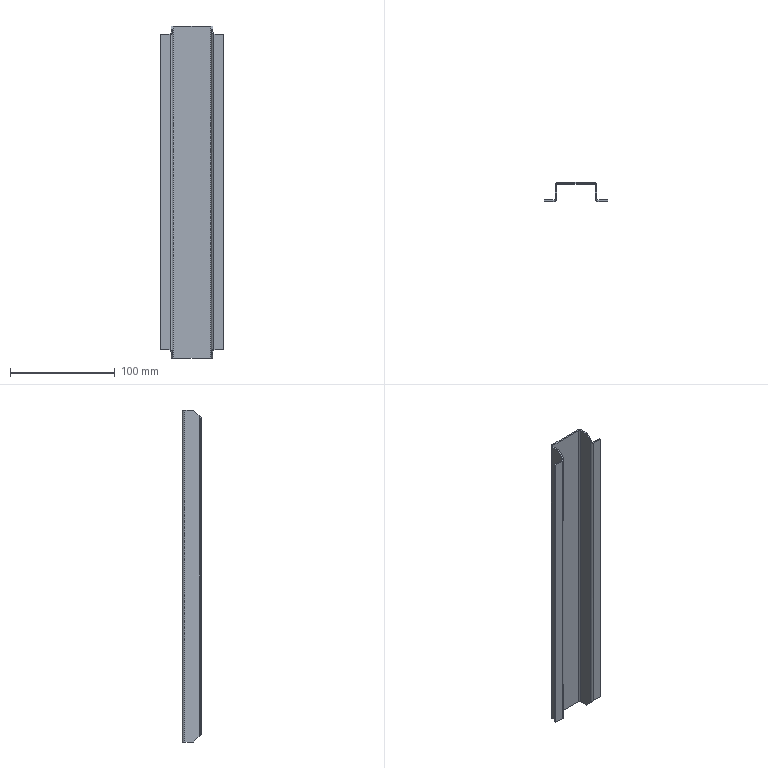Part | SolidWorks | features FlatPattern 1, ICE 1, SMBaseFlange 1, SheetMetal 1 | 1 solid | 42 faces | box 61 x 18.5 x 317 mm | volume 43080 mm3 | plane 30 | cylinder 8 | spline 4 | commonest cylinder face diameters 2 x4 5 x4
STEP:
#1=CARTESIAN_POINT('',(22.477,26.708,8.));
#2=VERTEX_POINT('',#1);
#3=CARTESIAN_POINT('',(12.977,26.708,8.));
#4=VERTEX_POINT('',#3);
#5=CARTESIAN_POINT('',(168.477,26.708,8.));
#6=DIRECTION('',(-1.,0.,0.));
#7=VECTOR('',#6,1000.);
#8=LINE('',#5,#7);
#9=EDGE_CURVE('',#2,#4,#8,.T.);
#10=ORIENTED_EDGE('',*,*,#9,.F.);
#11=CARTESIAN_POINT('',(22.477,26.708,309.));
#12=VERTEX_POINT('',#11);
#13=CARTESIAN_POINT('',(22.477,26.708,317.));
#14=DIRECTION('',(0.,0.,-1.));
#15=VECTOR('',#14,1000.);
#16=LINE('',#13,#15);
#17=EDGE_CURVE('',#12,#2,#16,.T.);
#18=ORIENTED_EDGE('',*,*,#17,.F.);
#19=CARTESIAN_POINT('',(12.977,26.708,309.));
#20=VERTEX_POINT('',#19);
#21=CARTESIAN_POINT('',(168.477,26.708,309.));
#22=DIRECTION('',(-1.,0.,0.));
#23=VECTOR('',#22,1000.);
#24=LINE('',#21,#23);
#25=EDGE_CURVE('',#12,#20,#24,.T.);
#26=ORIENTED_EDGE('',*,*,#25,.T.);
#27=CARTESIAN_POINT('',(12.977,26.708,317.));
#28=DIRECTION('',(0.,0.,-1.));
#29=VECTOR('',#28,1000.);
#30=LINE('',#27,#29);
#31=EDGE_CURVE('',#20,#4,#30,.T.);
#32=ORIENTED_EDGE('',*,*,#31,.T.);
#33=EDGE_LOOP('',(#10,#18,#26,#32));
#34=FACE_OUTER_BOUND('',#33,.T.);
#35=CARTESIAN_POINT('',(11.977,26.708,317.));
#36=DIRECTION('',(0.,1.,0.));
#37=DIRECTION('',(0.,0.,1.));
#38=AXIS2_PLACEMENT_3D('',#35,#36,#37);
#39=PLANE('',#38);
#40=ADVANCED_FACE('',(#34),#39,.F.);
#41=ORIENTED_EDGE('',*,*,#17,.T.);
#42=CARTESIAN_POINT('',(22.477,28.208,8.));
#43=VERTEX_POINT('',#42);
#44=CARTESIAN_POINT('',(22.477,26.708,8.));
#45=DIRECTION('',(0.,1.,0.));
#46=VECTOR('',#45,1000.);
#47=LINE('',#44,#46);
#48=EDGE_CURVE('',#2,#43,#47,.T.);
#49=ORIENTED_EDGE('',*,*,#48,.T.);
#50=CARTESIAN_POINT('',(22.477,28.208,309.));
#51=VERTEX_POINT('',#50);
#52=CARTESIAN_POINT('',(22.477,28.208,317.));
#53=DIRECTION('',(0.,0.,-1.));
#54=VECTOR('',#53,1000.);
#55=LINE('',#52,#54);
#56=EDGE_CURVE('',#51,#43,#55,.T.);
#57=ORIENTED_EDGE('',*,*,#56,.F.);
#58=CARTESIAN_POINT('',(22.477,26.708,309.));
#59=DIRECTION('',(0.,1.,0.));
#60=VECTOR('',#59,1000.);
#61=LINE('',#58,#60);
#62=EDGE_CURVE('',#12,#51,#61,.T.);
#63=ORIENTED_EDGE('',*,*,#62,.F.);
#64=EDGE_LOOP('',(#41,#49,#57,#63));
#65=FACE_OUTER_BOUND('',#64,.T.);
#66=CARTESIAN_POINT('',(22.477,28.208,317.));
#67=DIRECTION('',(1.,0.,0.));
#68=DIRECTION('',(0.,0.,-1.));
#69=AXIS2_PLACEMENT_3D('',#66,#67,#68);
#70=PLANE('',#69);
#71=ADVANCED_FACE('',(#65),#70,.T.);
#72=ORIENTED_EDGE('',*,*,#56,.T.);
#73=CARTESIAN_POINT('',(12.977,28.208,8.));
#74=VERTEX_POINT('',#73);
#75=CARTESIAN_POINT('',(11.977,28.208,8.));
#76=DIRECTION('',(-1.,0.,0.));
#77=VECTOR('',#76,1000.);
#78=LINE('',#75,#77);
#79=EDGE_CURVE('',#43,#74,#78,.T.);
#80=ORIENTED_EDGE('',*,*,#79,.T.);
#81=CARTESIAN_POINT('',(12.977,28.208,309.));
#82=VERTEX_POINT('',#81);
#83=CARTESIAN_POINT('',(12.977,28.208,317.));
#84=DIRECTION('',(0.,0.,-1.));
#85=VECTOR('',#84,1000.);
#86=LINE('',#83,#85);
#87=EDGE_CURVE('',#82,#74,#86,.T.);
#88=ORIENTED_EDGE('',*,*,#87,.F.);
#89=CARTESIAN_POINT('',(11.977,28.208,309.));
#90=DIRECTION('',(-1.,0.,0.));
#91=VECTOR('',#90,1000.);
#92=LINE('',#89,#91);
#93=EDGE_CURVE('',#51,#82,#92,.T.);
#94=ORIENTED_EDGE('',*,*,#93,.F.);
#95=EDGE_LOOP('',(#72,#80,#88,#94));
#96=FACE_OUTER_BOUND('',#95,.T.);
#97=CARTESIAN_POINT('',(11.977,28.208,317.));
#98=DIRECTION('',(0.,1.,0.));
#99=DIRECTION('',(0.,0.,1.));
#100=AXIS2_PLACEMENT_3D('',#97,#98,#99);
#101=PLANE('',#100);
#102=ADVANCED_FACE('',(#96),#101,.T.);
#103=ORIENTED_EDGE('',*,*,#87,.T.);
#104=CARTESIAN_POINT('',(11.977,29.208,5.5));
#105=VERTEX_POINT('',#104);
#106=CARTESIAN_POINT('',(11.977,29.208,5.5));
#107=CARTESIAN_POINT('',(11.977,28.623,6.964));
#108=CARTESIAN_POINT('',(12.391,28.208,8.));
#109=CARTESIAN_POINT('',(12.977,28.208,8.));
#110=(BOUNDED_CURVE()B_SPLINE_CURVE(3,(#106,#107,#108,#109),.UNSPECIFIED.,.F.,.F.)B_SPLINE_CURVE_WITH_KNOTS((4,4),(1.571,3.142),.UNSPECIFIED.)CURVE()GEOMETRIC_REPRESENTATION_ITEM()RATIONAL_B_SPLINE_CURVE((1.,0.8047,0.8047,1.))REPRESENTATION_ITEM(''));
#111=EDGE_CURVE('',#105,#74,#110,.T.);
#112=ORIENTED_EDGE('',*,*,#111,.F.);
#113=CARTESIAN_POINT('',(11.977,29.208,311.5));
#114=VERTEX_POINT('',#113);
#115=CARTESIAN_POINT('',(11.977,29.208,317.));
#116=DIRECTION('',(0.,0.,-1.));
#117=VECTOR('',#116,1000.);
#118=LINE('',#115,#117);
#119=EDGE_CURVE('',#114,#105,#118,.T.);
#120=ORIENTED_EDGE('',*,*,#119,.F.);
#121=CARTESIAN_POINT('',(12.977,28.208,309.));
#122=CARTESIAN_POINT('',(12.391,28.208,309.));
#123=CARTESIAN_POINT('',(11.977,28.623,310.036));
#124=CARTESIAN_POINT('',(11.977,29.208,311.5));
#125=(BOUNDED_CURVE()B_SPLINE_CURVE(3,(#121,#122,#123,#124),.UNSPECIFIED.,.F.,.F.)B_SPLINE_CURVE_WITH_KNOTS((4,4),(0.,1.571),.UNSPECIFIED.)CURVE()GEOMETRIC_REPRESENTATION_ITEM()RATIONAL_B_SPLINE_CURVE((1.,0.8047,0.8047,1.))REPRESENTATION_ITEM(''));
#126=EDGE_CURVE('',#82,#114,#125,.T.);
#127=ORIENTED_EDGE('',*,*,#126,.F.);
#128=EDGE_LOOP('',(#103,#112,#120,#127));
#129=FACE_OUTER_BOUND('',#128,.T.);
#130=CARTESIAN_POINT('',(12.977,29.208,317.));
#131=DIRECTION('',(0.,0.,-1.));
#132=DIRECTION('',(-1.,0.,0.));
#133=AXIS2_PLACEMENT_3D('',#130,#131,#132);
#134=CYLINDRICAL_SURFACE('',#133,1.);
#135=ADVANCED_FACE('',(#129),#134,.F.);
#136=ORIENTED_EDGE('',*,*,#119,.T.);
#137=CARTESIAN_POINT('',(11.977,34.708,0.));
#138=VERTEX_POINT('',#137);
#139=CARTESIAN_POINT('',(11.977,-118.542,153.25));
#140=DIRECTION('',(0.,-0.7071,0.7071));
#141=VECTOR('',#140,1000.);
#142=LINE('',#139,#141);
#143=EDGE_CURVE('',#138,#105,#142,.T.);
#144=ORIENTED_EDGE('',*,*,#143,.F.);
#145=CARTESIAN_POINT('',(11.977,42.708,0.));
#146=VERTEX_POINT('',#145);
#147=CARTESIAN_POINT('',(11.977,45.208,0.));
#148=DIRECTION('',(0.,-1.,0.));
#149=VECTOR('',#148,1000.);
#150=LINE('',#147,#149);
#151=EDGE_CURVE('',#146,#138,#150,.T.);
#152=ORIENTED_EDGE('',*,*,#151,.F.);
#153=CARTESIAN_POINT('',(11.977,42.708,317.));
#154=VERTEX_POINT('',#153);
#155=CARTESIAN_POINT('',(11.977,42.708,317.));
#156=DIRECTION('',(0.,0.,-1.));
#157=VECTOR('',#156,1000.);
#158=LINE('',#155,#157);
#159=EDGE_CURVE('',#154,#146,#158,.T.);
#160=ORIENTED_EDGE('',*,*,#159,.F.);
#161=CARTESIAN_POINT('',(11.977,34.708,317.));
#162=VERTEX_POINT('',#161);
#163=CARTESIAN_POINT('',(11.977,45.208,317.));
#164=DIRECTION('',(0.,-1.,0.));
#165=VECTOR('',#164,1000.);
#166=LINE('',#163,#165);
#167=EDGE_CURVE('',#154,#162,#166,.T.);
#168=ORIENTED_EDGE('',*,*,#167,.T.);
#169=CARTESIAN_POINT('',(11.977,39.958,322.25));
#170=DIRECTION('',(0.,0.7071,0.7071));
#171=VECTOR('',#170,1000.);
#172=LINE('',#169,#171);
#173=EDGE_CURVE('',#114,#162,#172,.T.);
#174=ORIENTED_EDGE('',*,*,#173,.F.);
#175=EDGE_LOOP('',(#136,#144,#152,#160,#168,#174));
#176=FACE_OUTER_BOUND('',#175,.T.);
#177=CARTESIAN_POINT('',(11.977,45.208,317.));
#178=DIRECTION('',(1.,0.,0.));
#179=DIRECTION('',(0.,0.,-1.));
#180=AXIS2_PLACEMENT_3D('',#177,#178,#179);
#181=PLANE('',#180);
#182=ADVANCED_FACE('',(#176),#181,.T.);
#183=CARTESIAN_POINT('',(10.477,34.708,0.));
#184=VERTEX_POINT('',#183);
#185=CARTESIAN_POINT('',(10.477,29.208,5.5));
#186=VERTEX_POINT('',#185);
#187=CARTESIAN_POINT('',(10.477,-118.542,153.25));
#188=DIRECTION('',(0.,-0.7071,0.7071));
#189=VECTOR('',#188,1000.);
#190=LINE('',#187,#189);
#191=EDGE_CURVE('',#184,#186,#190,.T.);
#192=ORIENTED_EDGE('',*,*,#191,.T.);
#193=CARTESIAN_POINT('',(10.477,29.208,311.5));
#194=VERTEX_POINT('',#193);
#195=CARTESIAN_POINT('',(10.477,29.208,317.));
#196=DIRECTION('',(0.,0.,-1.));
#197=VECTOR('',#196,1000.);
#198=LINE('',#195,#197);
#199=EDGE_CURVE('',#194,#186,#198,.T.);
#200=ORIENTED_EDGE('',*,*,#199,.F.);
#201=CARTESIAN_POINT('',(10.477,34.708,317.));
#202=VERTEX_POINT('',#201);
#203=CARTESIAN_POINT('',(10.477,39.958,322.25));
#204=DIRECTION('',(0.,0.7071,0.7071));
#205=VECTOR('',#204,1000.);
#206=LINE('',#203,#205);
#207=EDGE_CURVE('',#194,#202,#206,.T.);
#208=ORIENTED_EDGE('',*,*,#207,.T.);
#209=CARTESIAN_POINT('',(10.477,42.708,317.));
#210=VERTEX_POINT('',#209);
#211=CARTESIAN_POINT('',(10.477,45.208,317.));
#212=DIRECTION('',(0.,-1.,0.));
#213=VECTOR('',#212,1000.);
#214=LINE('',#211,#213);
#215=EDGE_CURVE('',#210,#202,#214,.T.);
#216=ORIENTED_EDGE('',*,*,#215,.F.);
#217=CARTESIAN_POINT('',(10.477,42.708,0.));
#218=VERTEX_POINT('',#217);
#219=CARTESIAN_POINT('',(10.477,42.708,317.));
#220=DIRECTION('',(0.,0.,-1.));
#221=VECTOR('',#220,1000.);
#222=LINE('',#219,#221);
#223=EDGE_CURVE('',#210,#218,#222,.T.);
#224=ORIENTED_EDGE('',*,*,#223,.T.);
#225=CARTESIAN_POINT('',(10.477,45.208,0.));
#226=DIRECTION('',(0.,-1.,0.));
#227=VECTOR('',#226,1000.);
#228=LINE('',#225,#227);
#229=EDGE_CURVE('',#218,#184,#228,.T.);
#230=ORIENTED_EDGE('',*,*,#229,.T.);
#231=EDGE_LOOP('',(#192,#200,#208,#216,#224,#230));
#232=FACE_OUTER_BOUND('',#231,.T.);
#233=CARTESIAN_POINT('',(10.477,45.208,317.));
#234=DIRECTION('',(1.,0.,0.));
#235=DIRECTION('',(0.,0.,-1.));
#236=AXIS2_PLACEMENT_3D('',#233,#234,#235);
#237=PLANE('',#236);
#238=ADVANCED_FACE('',(#232),#237,.F.);
#239=CARTESIAN_POINT('',(10.477,29.208,5.5));
#240=CARTESIAN_POINT('',(10.477,27.744,6.964));
#241=CARTESIAN_POINT('',(11.512,26.708,8.));
#242=CARTESIAN_POINT('',(12.977,26.708,8.));
#243=(BOUNDED_CURVE()B_SPLINE_CURVE(3,(#239,#240,#241,#242),.UNSPECIFIED.,.F.,.F.)B_SPLINE_CURVE_WITH_KNOTS((4,4),(1.571,3.142),.UNSPECIFIED.)CURVE()GEOMETRIC_REPRESENTATION_ITEM()RATIONAL_B_SPLINE_CURVE((1.,0.8047,0.8047,1.))REPRESENTATION_ITEM(''));
#244=EDGE_CURVE('',#186,#4,#243,.T.);
#245=ORIENTED_EDGE('',*,*,#244,.T.);
#246=ORIENTED_EDGE('',*,*,#31,.F.);
#247=CARTESIAN_POINT('',(12.977,26.708,309.));
#248=CARTESIAN_POINT('',(11.512,26.708,309.));
#249=CARTESIAN_POINT('',(10.477,27.744,310.036));
#250=CARTESIAN_POINT('',(10.477,29.208,311.5));
#251=(BOUNDED_CURVE()B_SPLINE_CURVE(3,(#247,#248,#249,#250),.UNSPECIFIED.,.F.,.F.)B_SPLINE_CURVE_WITH_KNOTS((4,4),(0.,1.571),.UNSPECIFIED.)CURVE()GEOMETRIC_REPRESENTATION_ITEM()RATIONAL_B_SPLINE_CURVE((1.,0.8047,0.8047,1.))REPRESENTATION_ITEM(''));
#252=EDGE_CURVE('',#20,#194,#251,.T.);
#253=ORIENTED_EDGE('',*,*,#252,.T.);
#254=ORIENTED_EDGE('',*,*,#199,.T.);
#255=EDGE_LOOP('',(#245,#246,#253,#254));
#256=FACE_OUTER_BOUND('',#255,.T.);
#257=CARTESIAN_POINT('',(12.977,29.208,317.));
#258=DIRECTION('',(0.,0.,-1.));
#259=DIRECTION('',(-1.,0.,0.));
#260=AXIS2_PLACEMENT_3D('',#257,#258,#259);
#261=CYLINDRICAL_SURFACE('',#260,2.5);
#262=ADVANCED_FACE('',(#256),#261,.T.);
#263=CARTESIAN_POINT('',(-28.023,34.708,0.));
#264=VERTEX_POINT('',#263);
#265=CARTESIAN_POINT('',(-28.023,42.708,0.));
#266=VERTEX_POINT('',#265);
#267=CARTESIAN_POINT('',(-28.023,28.208,0.));
#268=DIRECTION('',(0.,1.,0.));
#269=VECTOR('',#268,1000.);
#270=LINE('',#267,#269);
#271=EDGE_CURVE('',#264,#266,#270,.T.);
#272=ORIENTED_EDGE('',*,*,#271,.F.);
#273=CARTESIAN_POINT('',(-28.023,29.208,5.5));
#274=VERTEX_POINT('',#273);
#275=CARTESIAN_POINT('',(-28.023,-127.042,161.75));
#276=DIRECTION('',(0.,0.7071,-0.7071));
#277=VECTOR('',#276,1000.);
#278=LINE('',#275,#277);
#279=EDGE_CURVE('',#274,#264,#278,.T.);
#280=ORIENTED_EDGE('',*,*,#279,.F.);
#281=CARTESIAN_POINT('',(-28.023,29.208,311.5));
#282=VERTEX_POINT('',#281);
#283=CARTESIAN_POINT('',(-28.023,29.208,317.));
#284=DIRECTION('',(0.,0.,-1.));
#285=VECTOR('',#284,1000.);
#286=LINE('',#283,#285);
#287=EDGE_CURVE('',#282,#274,#286,.T.);
#288=ORIENTED_EDGE('',*,*,#287,.F.);
#289=CARTESIAN_POINT('',(-28.023,34.708,317.));
#290=VERTEX_POINT('',#289);
#291=CARTESIAN_POINT('',(-28.023,31.458,313.75));
#292=DIRECTION('',(0.,-0.7071,-0.7071));
#293=VECTOR('',#292,1000.);
#294=LINE('',#291,#293);
#295=EDGE_CURVE('',#290,#282,#294,.T.);
#296=ORIENTED_EDGE('',*,*,#295,.F.);
#297=CARTESIAN_POINT('',(-28.023,42.708,317.));
#298=VERTEX_POINT('',#297);
#299=CARTESIAN_POINT('',(-28.023,28.208,317.));
#300=DIRECTION('',(0.,1.,0.));
#301=VECTOR('',#300,1000.);
#302=LINE('',#299,#301);
#303=EDGE_CURVE('',#290,#298,#302,.T.);
#304=ORIENTED_EDGE('',*,*,#303,.T.);
#305=CARTESIAN_POINT('',(-28.023,42.708,317.));
#306=DIRECTION('',(0.,0.,-1.));
#307=VECTOR('',#306,1000.);
#308=LINE('',#305,#307);
#309=EDGE_CURVE('',#298,#266,#308,.T.);
#310=ORIENTED_EDGE('',*,*,#309,.T.);
#311=EDGE_LOOP('',(#272,#280,#288,#296,#304,#310));
#312=FACE_OUTER_BOUND('',#311,.T.);
#313=CARTESIAN_POINT('',(-28.023,28.208,317.));
#314=DIRECTION('',(-1.,0.,0.));
#315=DIRECTION('',(0.,0.,1.));
#316=AXIS2_PLACEMENT_3D('',#313,#314,#315);
#317=PLANE('',#316);
#318=ADVANCED_FACE('',(#312),#317,.T.);
#319=ORIENTED_EDGE('',*,*,#287,.T.);
#320=CARTESIAN_POINT('',(-29.023,28.208,8.));
#321=VERTEX_POINT('',#320);
#322=CARTESIAN_POINT('',(-29.023,28.208,8.));
#323=CARTESIAN_POINT('',(-28.437,28.208,8.));
#324=CARTESIAN_POINT('',(-28.023,28.623,6.964));
#325=CARTESIAN_POINT('',(-28.023,29.208,5.5));
#326=(BOUNDED_CURVE()B_SPLINE_CURVE(3,(#322,#323,#324,#325),.UNSPECIFIED.,.F.,.F.)B_SPLINE_CURVE_WITH_KNOTS((4,4),(3.142,4.712),.UNSPECIFIED.)CURVE()GEOMETRIC_REPRESENTATION_ITEM()RATIONAL_B_SPLINE_CURVE((1.,0.8047,0.8047,1.))REPRESENTATION_ITEM(''));
#327=EDGE_CURVE('',#321,#274,#326,.T.);
#328=ORIENTED_EDGE('',*,*,#327,.F.);
#329=CARTESIAN_POINT('',(-29.023,28.208,309.));
#330=VERTEX_POINT('',#329);
#331=CARTESIAN_POINT('',(-29.023,28.208,317.));
#332=DIRECTION('',(0.,0.,-1.));
#333=VECTOR('',#332,1000.);
#334=LINE('',#331,#333);
#335=EDGE_CURVE('',#330,#321,#334,.T.);
#336=ORIENTED_EDGE('',*,*,#335,.F.);
#337=CARTESIAN_POINT('',(-28.023,29.208,311.5));
#338=CARTESIAN_POINT('',(-28.023,28.623,310.036));
#339=CARTESIAN_POINT('',(-28.437,28.208,309.));
#340=CARTESIAN_POINT('',(-29.023,28.208,309.));
#341=(BOUNDED_CURVE()B_SPLINE_CURVE(3,(#337,#338,#339,#340),.UNSPECIFIED.,.F.,.F.)B_SPLINE_CURVE_WITH_KNOTS((4,4),(4.712,6.283),.UNSPECIFIED.)CURVE()GEOMETRIC_REPRESENTATION_ITEM()RATIONAL_B_SPLINE_CURVE((1.,0.8047,0.8047,1.))REPRESENTATION_ITEM(''));
#342=EDGE_CURVE('',#282,#330,#341,.T.);
#343=ORIENTED_EDGE('',*,*,#342,.F.);
#344=EDGE_LOOP('',(#319,#328,#336,#343));
#345=FACE_OUTER_BOUND('',#344,.T.);
#346=CARTESIAN_POINT('',(-29.023,29.208,317.));
#347=DIRECTION('',(0.,0.,-1.));
#348=DIRECTION('',(-1.,0.,0.));
#349=AXIS2_PLACEMENT_3D('',#346,#347,#348);
#350=CYLINDRICAL_SURFACE('',#349,1.);
#351=ADVANCED_FACE('',(#345),#350,.F.);
#352=ORIENTED_EDGE('',*,*,#335,.T.);
#353=CARTESIAN_POINT('',(-38.523,28.208,8.));
#354=VERTEX_POINT('',#353);
#355=CARTESIAN_POINT('',(-38.523,28.208,8.));
#356=DIRECTION('',(-1.,0.,0.));
#357=VECTOR('',#356,1000.);
#358=LINE('',#355,#357);
#359=EDGE_CURVE('',#321,#354,#358,.T.);
#360=ORIENTED_EDGE('',*,*,#359,.T.);
#361=CARTESIAN_POINT('',(-38.523,28.208,309.));
#362=VERTEX_POINT('',#361);
#363=CARTESIAN_POINT('',(-38.523,28.208,317.));
#364=DIRECTION('',(0.,0.,-1.));
#365=VECTOR('',#364,1000.);
#366=LINE('',#363,#365);
#367=EDGE_CURVE('',#362,#354,#366,.T.);
#368=ORIENTED_EDGE('',*,*,#367,.F.);
#369=CARTESIAN_POINT('',(-38.523,28.208,309.));
#370=DIRECTION('',(-1.,0.,0.));
#371=VECTOR('',#370,1000.);
#372=LINE('',#369,#371);
#373=EDGE_CURVE('',#330,#362,#372,.T.);
#374=ORIENTED_EDGE('',*,*,#373,.F.);
#375=EDGE_LOOP('',(#352,#360,#368,#374));
#376=FACE_OUTER_BOUND('',#375,.T.);
#377=CARTESIAN_POINT('',(-38.523,28.208,317.));
#378=DIRECTION('',(0.,1.,0.));
#379=DIRECTION('',(0.,0.,1.));
#380=AXIS2_PLACEMENT_3D('',#377,#378,#379);
#381=PLANE('',#380);
#382=ADVANCED_FACE('',(#376),#381,.T.);
#383=ORIENTED_EDGE('',*,*,#367,.T.);
#384=CARTESIAN_POINT('',(-38.523,26.708,8.));
#385=VERTEX_POINT('',#384);
#386=CARTESIAN_POINT('',(-38.523,26.708,8.));
#387=DIRECTION('',(0.,1.,0.));
#388=VECTOR('',#387,1000.);
#389=LINE('',#386,#388);
#390=EDGE_CURVE('',#385,#354,#389,.T.);
#391=ORIENTED_EDGE('',*,*,#390,.F.);
#392=CARTESIAN_POINT('',(-38.523,26.708,309.));
#393=VERTEX_POINT('',#392);
#394=CARTESIAN_POINT('',(-38.523,26.708,317.));
#395=DIRECTION('',(0.,0.,-1.));
#396=VECTOR('',#395,1000.);
#397=LINE('',#394,#396);
#398=EDGE_CURVE('',#393,#385,#397,.T.);
#399=ORIENTED_EDGE('',*,*,#398,.F.);
#400=CARTESIAN_POINT('',(-38.523,26.708,309.));
#401=DIRECTION('',(0.,1.,0.));
#402=VECTOR('',#401,1000.);
#403=LINE('',#400,#402);
#404=EDGE_CURVE('',#393,#362,#403,.T.);
#405=ORIENTED_EDGE('',*,*,#404,.T.);
#406=EDGE_LOOP('',(#383,#391,#399,#405));
#407=FACE_OUTER_BOUND('',#406,.T.);
#408=CARTESIAN_POINT('',(-38.523,26.708,317.));
#409=DIRECTION('',(-1.,0.,0.));
#410=DIRECTION('',(0.,0.,1.));
#411=AXIS2_PLACEMENT_3D('',#408,#409,#410);
#412=PLANE('',#411);
#413=ADVANCED_FACE('',(#407),#412,.T.);
#414=CARTESIAN_POINT('',(-29.023,26.708,8.));
#415=VERTEX_POINT('',#414);
#416=CARTESIAN_POINT('',(168.477,26.708,8.));
#417=DIRECTION('',(-1.,0.,0.));
#418=VECTOR('',#417,1000.);
#419=LINE('',#416,#418);
#420=EDGE_CURVE('',#415,#385,#419,.T.);
#421=ORIENTED_EDGE('',*,*,#420,.F.);
#422=CARTESIAN_POINT('',(-29.023,26.708,309.));
#423=VERTEX_POINT('',#422);
#424=CARTESIAN_POINT('',(-29.023,26.708,317.));
#425=DIRECTION('',(0.,0.,-1.));
#426=VECTOR('',#425,1000.);
#427=LINE('',#424,#426);
#428=EDGE_CURVE('',#423,#415,#427,.T.);
#429=ORIENTED_EDGE('',*,*,#428,.F.);
#430=CARTESIAN_POINT('',(168.477,26.708,309.));
#431=DIRECTION('',(-1.,0.,0.));
#432=VECTOR('',#431,1000.);
#433=LINE('',#430,#432);
#434=EDGE_CURVE('',#423,#393,#433,.T.);
#435=ORIENTED_EDGE('',*,*,#434,.T.);
#436=ORIENTED_EDGE('',*,*,#398,.T.);
#437=EDGE_LOOP('',(#421,#429,#435,#436));
#438=FACE_OUTER_BOUND('',#437,.T.);
#439=CARTESIAN_POINT('',(-38.523,26.708,317.));
#440=DIRECTION('',(0.,1.,0.));
#441=DIRECTION('',(0.,0.,1.));
#442=AXIS2_PLACEMENT_3D('',#439,#440,#441);
#443=PLANE('',#442);
#444=ADVANCED_FACE('',(#438),#443,.F.);
#445=CARTESIAN_POINT('',(-26.523,29.208,5.5));
#446=VERTEX_POINT('',#445);
#447=CARTESIAN_POINT('',(-29.023,26.708,8.));
#448=CARTESIAN_POINT('',(-27.559,26.708,8.));
#449=CARTESIAN_POINT('',(-26.523,27.744,6.964));
#450=CARTESIAN_POINT('',(-26.523,29.208,5.5));
#451=(BOUNDED_CURVE()B_SPLINE_CURVE(3,(#447,#448,#449,#450),.UNSPECIFIED.,.F.,.T.)B_SPLINE_CURVE_WITH_KNOTS((4,4),(3.142,4.712),.UNSPECIFIED.)CURVE()GEOMETRIC_REPRESENTATION_ITEM()RATIONAL_B_SPLINE_CURVE((1.,0.8047,0.8047,1.))REPRESENTATION_ITEM(''));
#452=EDGE_CURVE('',#415,#446,#451,.T.);
#453=ORIENTED_EDGE('',*,*,#452,.T.);
#454=CARTESIAN_POINT('',(-26.523,29.208,311.5));
#455=VERTEX_POINT('',#454);
#456=CARTESIAN_POINT('',(-26.523,29.208,317.));
#457=DIRECTION('',(0.,0.,-1.));
#458=VECTOR('',#457,1000.);
#459=LINE('',#456,#458);
#460=EDGE_CURVE('',#455,#446,#459,.T.);
#461=ORIENTED_EDGE('',*,*,#460,.F.);
#462=CARTESIAN_POINT('',(-26.523,29.208,311.5));
#463=CARTESIAN_POINT('',(-26.523,27.744,310.036));
#464=CARTESIAN_POINT('',(-27.559,26.708,309.));
#465=CARTESIAN_POINT('',(-29.023,26.708,309.));
#466=(BOUNDED_CURVE()B_SPLINE_CURVE(3,(#462,#463,#464,#465),.UNSPECIFIED.,.F.,.F.)B_SPLINE_CURVE_WITH_KNOTS((4,4),(4.712,6.283),.UNSPECIFIED.)CURVE()GEOMETRIC_REPRESENTATION_ITEM()RATIONAL_B_SPLINE_CURVE((1.,0.8047,0.8047,1.))REPRESENTATION_ITEM(''));
#467=EDGE_CURVE('',#455,#423,#466,.T.);
#468=ORIENTED_EDGE('',*,*,#467,.T.);
#469=ORIENTED_EDGE('',*,*,#428,.T.);
#470=EDGE_LOOP('',(#453,#461,#468,#469));
#471=FACE_OUTER_BOUND('',#470,.T.);
#472=CARTESIAN_POINT('',(-29.023,29.208,317.));
#473=DIRECTION('',(0.,0.,-1.));
#474=DIRECTION('',(-1.,0.,0.));
#475=AXIS2_PLACEMENT_3D('',#472,#473,#474);
#476=CYLINDRICAL_SURFACE('',#475,2.5);
#477=ADVANCED_FACE('',(#471),#476,.T.);
#478=CARTESIAN_POINT('',(-26.523,34.708,0.));
#479=VERTEX_POINT('',#478);
#480=CARTESIAN_POINT('',(-26.523,-127.042,161.75));
#481=DIRECTION('',(0.,0.7071,-0.7071));
#482=VECTOR('',#481,1000.);
#483=LINE('',#480,#482);
#484=EDGE_CURVE('',#446,#479,#483,.T.);
#485=ORIENTED_EDGE('',*,*,#484,.T.);
#486=CARTESIAN_POINT('',(-26.523,42.708,0.));
#487=VERTEX_POINT('',#486);
#488=CARTESIAN_POINT('',(-26.523,28.208,0.));
#489=DIRECTION('',(0.,1.,0.));
#490=VECTOR('',#489,1000.);
#491=LINE('',#488,#490);
#492=EDGE_CURVE('',#479,#487,#491,.T.);
#493=ORIENTED_EDGE('',*,*,#492,.T.);
#494=CARTESIAN_POINT('',(-26.523,42.708,317.));
#495=VERTEX_POINT('',#494);
#496=CARTESIAN_POINT('',(-26.523,42.708,317.));
#497=DIRECTION('',(0.,0.,-1.));
#498=VECTOR('',#497,1000.);
#499=LINE('',#496,#498);
#500=EDGE_CURVE('',#495,#487,#499,.T.);
#501=ORIENTED_EDGE('',*,*,#500,.F.);
#502=CARTESIAN_POINT('',(-26.523,34.708,317.));
#503=VERTEX_POINT('',#502);
#504=CARTESIAN_POINT('',(-26.523,28.208,317.));
#505=DIRECTION('',(0.,1.,0.));
#506=VECTOR('',#505,1000.);
#507=LINE('',#504,#506);
#508=EDGE_CURVE('',#503,#495,#507,.T.);
#509=ORIENTED_EDGE('',*,*,#508,.F.);
#510=CARTESIAN_POINT('',(-26.523,31.458,313.75));
#511=DIRECTION('',(0.,-0.7071,-0.7071));
#512=VECTOR('',#511,1000.);
#513=LINE('',#510,#512);
#514=EDGE_CURVE('',#503,#455,#513,.T.);
#515=ORIENTED_EDGE('',*,*,#514,.T.);
#516=ORIENTED_EDGE('',*,*,#460,.T.);
#517=EDGE_LOOP('',(#485,#493,#501,#509,#515,#516));
#518=FACE_OUTER_BOUND('',#517,.T.);
#519=CARTESIAN_POINT('',(-26.523,28.208,317.));
#520=DIRECTION('',(-1.,0.,0.));
#521=DIRECTION('',(0.,0.,1.));
#522=AXIS2_PLACEMENT_3D('',#519,#520,#521);
#523=PLANE('',#522);
#524=ADVANCED_FACE('',(#518),#523,.F.);
#525=ORIENTED_EDGE('',*,*,#303,.F.);
#526=CARTESIAN_POINT('',(-28.023,34.708,317.));
#527=DIRECTION('',(1.,0.,0.));
#528=VECTOR('',#527,1000.);
#529=LINE('',#526,#528);
#530=EDGE_CURVE('',#290,#503,#529,.T.);
#531=ORIENTED_EDGE('',*,*,#530,.T.);
#532=ORIENTED_EDGE('',*,*,#508,.T.);
#533=CARTESIAN_POINT('',(-26.523,42.708,317.));
#534=DIRECTION('',(-1.,0.,0.));
#535=VECTOR('',#534,1000.);
#536=LINE('',#533,#535);
#537=EDGE_CURVE('',#495,#298,#536,.T.);
#538=ORIENTED_EDGE('',*,*,#537,.T.);
#539=EDGE_LOOP('',(#525,#531,#532,#538));
#540=FACE_OUTER_BOUND('',#539,.T.);
#541=CARTESIAN_POINT('',(-29.023,26.708,317.));
#542=DIRECTION('',(0.,0.,1.));
#543=DIRECTION('',(1.,0.,0.));
#544=AXIS2_PLACEMENT_3D('',#541,#542,#543);
#545=PLANE('',#544);
#546=ADVANCED_FACE('',(#540),#545,.T.);
#547=CARTESIAN_POINT('',(-25.523,45.208,317.));
#548=VERTEX_POINT('',#547);
#549=CARTESIAN_POINT('',(-25.523,43.708,317.));
#550=VERTEX_POINT('',#549);
#551=CARTESIAN_POINT('',(-25.523,45.208,317.));
#552=DIRECTION('',(0.,-1.,0.));
#553=VECTOR('',#552,1000.);
#554=LINE('',#551,#553);
#555=EDGE_CURVE('',#548,#550,#554,.T.);
#556=ORIENTED_EDGE('',*,*,#555,.F.);
#557=CARTESIAN_POINT('',(-25.523,42.708,317.));
#558=DIRECTION('',(0.,0.,-1.));
#559=DIRECTION('',(1.,0.,0.));
#560=AXIS2_PLACEMENT_3D('',#557,#558,#559);
#561=CIRCLE('',#560,2.5);
#562=EDGE_CURVE('',#298,#548,#561,.T.);
#563=ORIENTED_EDGE('',*,*,#562,.F.);
#564=ORIENTED_EDGE('',*,*,#537,.F.);
#565=CARTESIAN_POINT('',(-25.523,42.708,317.));
#566=DIRECTION('',(0.,0.,-1.));
#567=DIRECTION('',(1.,0.,0.));
#568=AXIS2_PLACEMENT_3D('',#565,#566,#567);
#569=CIRCLE('',#568,1.);
#570=EDGE_CURVE('',#495,#550,#569,.T.);
#571=ORIENTED_EDGE('',*,*,#570,.T.);
#572=EDGE_LOOP('',(#556,#563,#564,#571));
#573=FACE_OUTER_BOUND('',#572,.T.);
#574=CARTESIAN_POINT('',(-25.523,45.208,317.));
#575=DIRECTION('',(0.,0.,1.));
#576=DIRECTION('',(1.,0.,0.));
#577=AXIS2_PLACEMENT_3D('',#574,#575,#576);
#578=PLANE('',#577);
#579=ADVANCED_FACE('',(#573),#578,.T.);
#580=CARTESIAN_POINT('',(9.477,45.208,317.));
#581=VERTEX_POINT('',#580);
#582=CARTESIAN_POINT('',(-28.023,45.208,317.));
#583=DIRECTION('',(1.,0.,0.));
#584=VECTOR('',#583,1000.);
#585=LINE('',#582,#584);
#586=EDGE_CURVE('',#548,#581,#585,.T.);
#587=ORIENTED_EDGE('',*,*,#586,.F.);
#588=ORIENTED_EDGE('',*,*,#555,.T.);
#589=CARTESIAN_POINT('',(9.477,43.708,317.));
#590=VERTEX_POINT('',#589);
#591=CARTESIAN_POINT('',(-28.023,43.708,317.));
#592=DIRECTION('',(1.,0.,0.));
#593=VECTOR('',#592,1000.);
#594=LINE('',#591,#593);
#595=EDGE_CURVE('',#550,#590,#594,.T.);
#596=ORIENTED_EDGE('',*,*,#595,.T.);
#597=CARTESIAN_POINT('',(9.477,43.708,317.));
#598=DIRECTION('',(0.,1.,0.));
#599=VECTOR('',#598,1000.);
#600=LINE('',#597,#599);
#601=EDGE_CURVE('',#590,#581,#600,.T.);
#602=ORIENTED_EDGE('',*,*,#601,.T.);
#603=EDGE_LOOP('',(#587,#588,#596,#602));
#604=FACE_OUTER_BOUND('',#603,.T.);
#605=CARTESIAN_POINT('',(-26.523,42.708,317.));
#606=DIRECTION('',(0.,0.,1.));
#607=DIRECTION('',(1.,0.,0.));
#608=AXIS2_PLACEMENT_3D('',#605,#606,#607);
#609=PLANE('',#608);
#610=ADVANCED_FACE('',(#604),#609,.T.);
#611=CARTESIAN_POINT('',(-28.023,42.708,0.));
#612=DIRECTION('',(1.,0.,0.));
#613=VECTOR('',#612,1000.);
#614=LINE('',#611,#613);
#615=EDGE_CURVE('',#266,#487,#614,.T.);
#616=ORIENTED_EDGE('',*,*,#615,.F.);
#617=CARTESIAN_POINT('',(-25.523,45.208,0.));
#618=VERTEX_POINT('',#617);
#619=CARTESIAN_POINT('',(-25.523,42.708,0.));
#620=DIRECTION('',(0.,0.,-1.));
#621=DIRECTION('',(1.,0.,0.));
#622=AXIS2_PLACEMENT_3D('',#619,#620,#621);
#623=CIRCLE('',#622,2.5);
#624=EDGE_CURVE('',#266,#618,#623,.T.);
#625=ORIENTED_EDGE('',*,*,#624,.T.);
#626=CARTESIAN_POINT('',(-25.523,43.708,0.));
#627=VERTEX_POINT('',#626);
#628=CARTESIAN_POINT('',(-25.523,43.708,0.));
#629=DIRECTION('',(0.,1.,0.));
#630=VECTOR('',#629,1000.);
#631=LINE('',#628,#630);
#632=EDGE_CURVE('',#627,#618,#631,.T.);
#633=ORIENTED_EDGE('',*,*,#632,.F.);
#634=CARTESIAN_POINT('',(-25.523,42.708,0.));
#635=DIRECTION('',(0.,0.,-1.));
#636=DIRECTION('',(1.,0.,0.));
#637=AXIS2_PLACEMENT_3D('',#634,#635,#636);
#638=CIRCLE('',#637,1.);
#639=EDGE_CURVE('',#487,#627,#638,.T.);
#640=ORIENTED_EDGE('',*,*,#639,.F.);
#641=EDGE_LOOP('',(#616,#625,#633,#640));
#642=FACE_OUTER_BOUND('',#641,.T.);
#643=CARTESIAN_POINT('',(-28.023,42.708,0.));
#644=DIRECTION('',(0.,0.,-1.));
#645=DIRECTION('',(-1.,0.,0.));
#646=AXIS2_PLACEMENT_3D('',#643,#644,#645);
#647=PLANE('',#646);
#648=ADVANCED_FACE('',(#642),#647,.T.);
#649=ORIENTED_EDGE('',*,*,#492,.F.);
#650=CARTESIAN_POINT('',(-28.023,34.708,0.));
#651=DIRECTION('',(1.,0.,0.));
#652=VECTOR('',#651,1000.);
#653=LINE('',#650,#652);
#654=EDGE_CURVE('',#264,#479,#653,.T.);
#655=ORIENTED_EDGE('',*,*,#654,.F.);
#656=ORIENTED_EDGE('',*,*,#271,.T.);
#657=ORIENTED_EDGE('',*,*,#615,.T.);
#658=EDGE_LOOP('',(#649,#655,#656,#657));
#659=FACE_OUTER_BOUND('',#658,.T.);
#660=CARTESIAN_POINT('',(-25.523,43.708,0.));
#661=DIRECTION('',(0.,0.,-1.));
#662=DIRECTION('',(-1.,0.,0.));
#663=AXIS2_PLACEMENT_3D('',#660,#661,#662);
#664=PLANE('',#663);
#665=ADVANCED_FACE('',(#659),#664,.T.);
#666=CARTESIAN_POINT('',(11.977,42.708,317.));
#667=DIRECTION('',(-1.,0.,0.));
#668=VECTOR('',#667,1000.);
#669=LINE('',#666,#668);
#670=EDGE_CURVE('',#154,#210,#669,.T.);
#671=ORIENTED_EDGE('',*,*,#670,.F.);
#672=CARTESIAN_POINT('',(9.477,42.708,317.));
#673=DIRECTION('',(0.,0.,-1.));
#674=DIRECTION('',(1.,0.,0.));
#675=AXIS2_PLACEMENT_3D('',#672,#673,#674);
#676=CIRCLE('',#675,2.5);
#677=EDGE_CURVE('',#581,#154,#676,.T.);
#678=ORIENTED_EDGE('',*,*,#677,.F.);
#679=ORIENTED_EDGE('',*,*,#601,.F.);
#680=CARTESIAN_POINT('',(9.477,42.708,317.));
#681=DIRECTION('',(0.,0.,-1.));
#682=DIRECTION('',(1.,0.,0.));
#683=AXIS2_PLACEMENT_3D('',#680,#681,#682);
#684=CIRCLE('',#683,1.);
#685=EDGE_CURVE('',#590,#210,#684,.T.);
#686=ORIENTED_EDGE('',*,*,#685,.T.);
#687=EDGE_LOOP('',(#671,#678,#679,#686));
#688=FACE_OUTER_BOUND('',#687,.T.);
#689=CARTESIAN_POINT('',(11.977,42.708,317.));
#690=DIRECTION('',(0.,0.,1.));
#691=DIRECTION('',(1.,0.,0.));
#692=AXIS2_PLACEMENT_3D('',#689,#690,#691);
#693=PLANE('',#692);
#694=ADVANCED_FACE('',(#688),#693,.T.);
#695=ORIENTED_EDGE('',*,*,#215,.T.);
#696=CARTESIAN_POINT('',(10.477,34.708,317.));
#697=DIRECTION('',(1.,0.,0.));
#698=VECTOR('',#697,1000.);
#699=LINE('',#696,#698);
#700=EDGE_CURVE('',#202,#162,#699,.T.);
#701=ORIENTED_EDGE('',*,*,#700,.T.);
#702=ORIENTED_EDGE('',*,*,#167,.F.);
#703=ORIENTED_EDGE('',*,*,#670,.T.);
#704=EDGE_LOOP('',(#695,#701,#702,#703));
#705=FACE_OUTER_BOUND('',#704,.T.);
#706=CARTESIAN_POINT('',(9.477,43.708,317.));
#707=DIRECTION('',(0.,0.,1.));
#708=DIRECTION('',(1.,0.,0.));
#709=AXIS2_PLACEMENT_3D('',#706,#707,#708);
#710=PLANE('',#709);
#711=ADVANCED_FACE('',(#705),#710,.T.);
#712=CARTESIAN_POINT('',(9.477,45.208,0.));
#713=VERTEX_POINT('',#712);
#714=CARTESIAN_POINT('',(9.477,43.708,0.));
#715=VERTEX_POINT('',#714);
#716=CARTESIAN_POINT('',(9.477,45.208,0.));
#717=DIRECTION('',(0.,-1.,0.));
#718=VECTOR('',#717,1000.);
#719=LINE('',#716,#718);
#720=EDGE_CURVE('',#713,#715,#719,.T.);
#721=ORIENTED_EDGE('',*,*,#720,.F.);
#722=CARTESIAN_POINT('',(9.477,42.708,0.));
#723=DIRECTION('',(0.,0.,-1.));
#724=DIRECTION('',(1.,0.,0.));
#725=AXIS2_PLACEMENT_3D('',#722,#723,#724);
#726=CIRCLE('',#725,2.5);
#727=EDGE_CURVE('',#713,#146,#726,.T.);
#728=ORIENTED_EDGE('',*,*,#727,.T.);
#729=CARTESIAN_POINT('',(10.477,42.708,0.));
#730=DIRECTION('',(1.,0.,0.));
#731=VECTOR('',#730,1000.);
#732=LINE('',#729,#731);
#733=EDGE_CURVE('',#218,#146,#732,.T.);
#734=ORIENTED_EDGE('',*,*,#733,.F.);
#735=CARTESIAN_POINT('',(9.477,42.708,0.));
#736=DIRECTION('',(0.,0.,-1.));
#737=DIRECTION('',(1.,0.,0.));
#738=AXIS2_PLACEMENT_3D('',#735,#736,#737);
#739=CIRCLE('',#738,1.);
#740=EDGE_CURVE('',#715,#218,#739,.T.);
#741=ORIENTED_EDGE('',*,*,#740,.F.);
#742=EDGE_LOOP('',(#721,#728,#734,#741));
#743=FACE_OUTER_BOUND('',#742,.T.);
#744=CARTESIAN_POINT('',(9.477,45.208,0.));
#745=DIRECTION('',(0.,0.,-1.));
#746=DIRECTION('',(-1.,0.,0.));
#747=AXIS2_PLACEMENT_3D('',#744,#745,#746);
#748=PLANE('',#747);
#749=ADVANCED_FACE('',(#743),#748,.T.);
#750=CARTESIAN_POINT('',(-28.023,45.208,0.));
#751=DIRECTION('',(1.,0.,0.));
#752=VECTOR('',#751,1000.);
#753=LINE('',#750,#752);
#754=EDGE_CURVE('',#618,#713,#753,.T.);
#755=ORIENTED_EDGE('',*,*,#754,.T.);
#756=ORIENTED_EDGE('',*,*,#720,.T.);
#757=CARTESIAN_POINT('',(-28.023,43.708,0.));
#758=DIRECTION('',(1.,0.,0.));
#759=VECTOR('',#758,1000.);
#760=LINE('',#757,#759);
#761=EDGE_CURVE('',#627,#715,#760,.T.);
#762=ORIENTED_EDGE('',*,*,#761,.F.);
#763=ORIENTED_EDGE('',*,*,#632,.T.);
#764=EDGE_LOOP('',(#755,#756,#762,#763));
#765=FACE_OUTER_BOUND('',#764,.T.);
#766=CARTESIAN_POINT('',(10.477,42.708,0.));
#767=DIRECTION('',(0.,0.,-1.));
#768=DIRECTION('',(-1.,0.,0.));
#769=AXIS2_PLACEMENT_3D('',#766,#767,#768);
#770=PLANE('',#769);
#771=ADVANCED_FACE('',(#765),#770,.T.);
#772=ORIENTED_EDGE('',*,*,#151,.T.);
#773=CARTESIAN_POINT('',(11.977,34.708,0.));
#774=DIRECTION('',(-1.,0.,0.));
#775=VECTOR('',#774,1000.);
#776=LINE('',#773,#775);
#777=EDGE_CURVE('',#138,#184,#776,.T.);
#778=ORIENTED_EDGE('',*,*,#777,.T.);
#779=ORIENTED_EDGE('',*,*,#229,.F.);
#780=ORIENTED_EDGE('',*,*,#733,.T.);
#781=EDGE_LOOP('',(#772,#778,#779,#780));
#782=FACE_OUTER_BOUND('',#781,.T.);
#783=CARTESIAN_POINT('',(12.977,26.708,0.));
#784=DIRECTION('',(0.,0.,-1.));
#785=DIRECTION('',(-1.,0.,0.));
#786=AXIS2_PLACEMENT_3D('',#783,#784,#785);
#787=PLANE('',#786);
#788=ADVANCED_FACE('',(#782),#787,.T.);
#789=ORIENTED_EDGE('',*,*,#727,.F.);
#790=CARTESIAN_POINT('',(9.477,45.208,317.));
#791=DIRECTION('',(0.,0.,-1.));
#792=VECTOR('',#791,1000.);
#793=LINE('',#790,#792);
#794=EDGE_CURVE('',#581,#713,#793,.T.);
#795=ORIENTED_EDGE('',*,*,#794,.F.);
#796=ORIENTED_EDGE('',*,*,#677,.T.);
#797=ORIENTED_EDGE('',*,*,#159,.T.);
#798=EDGE_LOOP('',(#789,#795,#796,#797));
#799=FACE_OUTER_BOUND('',#798,.T.);
#800=CARTESIAN_POINT('',(9.477,42.708,317.));
#801=DIRECTION('',(0.,0.,-1.));
#802=DIRECTION('',(-1.,0.,0.));
#803=AXIS2_PLACEMENT_3D('',#800,#801,#802);
#804=CYLINDRICAL_SURFACE('',#803,2.5);
#805=ADVANCED_FACE('',(#799),#804,.T.);
#806=ORIENTED_EDGE('',*,*,#754,.F.);
#807=CARTESIAN_POINT('',(-25.523,45.208,317.));
#808=DIRECTION('',(0.,0.,-1.));
#809=VECTOR('',#808,1000.);
#810=LINE('',#807,#809);
#811=EDGE_CURVE('',#548,#618,#810,.T.);
#812=ORIENTED_EDGE('',*,*,#811,.F.);
#813=ORIENTED_EDGE('',*,*,#586,.T.);
#814=ORIENTED_EDGE('',*,*,#794,.T.);
#815=EDGE_LOOP('',(#806,#812,#813,#814));
#816=FACE_OUTER_BOUND('',#815,.T.);
#817=CARTESIAN_POINT('',(-28.023,45.208,317.));
#818=DIRECTION('',(0.,1.,0.));
#819=DIRECTION('',(0.,0.,1.));
#820=AXIS2_PLACEMENT_3D('',#817,#818,#819);
#821=PLANE('',#820);
#822=ADVANCED_FACE('',(#816),#821,.T.);
#823=ORIENTED_EDGE('',*,*,#624,.F.);
#824=ORIENTED_EDGE('',*,*,#309,.F.);
#825=ORIENTED_EDGE('',*,*,#562,.T.);
#826=ORIENTED_EDGE('',*,*,#811,.T.);
#827=EDGE_LOOP('',(#823,#824,#825,#826));
#828=FACE_OUTER_BOUND('',#827,.T.);
#829=CARTESIAN_POINT('',(-25.523,42.708,317.));
#830=DIRECTION('',(0.,0.,-1.));
#831=DIRECTION('',(-1.,0.,0.));
#832=AXIS2_PLACEMENT_3D('',#829,#830,#831);
#833=CYLINDRICAL_SURFACE('',#832,2.5);
#834=ADVANCED_FACE('',(#828),#833,.T.);
#835=ORIENTED_EDGE('',*,*,#639,.T.);
#836=CARTESIAN_POINT('',(-25.523,43.708,317.));
#837=DIRECTION('',(0.,0.,-1.));
#838=VECTOR('',#837,1000.);
#839=LINE('',#836,#838);
#840=EDGE_CURVE('',#550,#627,#839,.T.);
#841=ORIENTED_EDGE('',*,*,#840,.F.);
#842=ORIENTED_EDGE('',*,*,#570,.F.);
#843=ORIENTED_EDGE('',*,*,#500,.T.);
#844=EDGE_LOOP('',(#835,#841,#842,#843));
#845=FACE_OUTER_BOUND('',#844,.T.);
#846=CARTESIAN_POINT('',(-25.523,42.708,317.));
#847=DIRECTION('',(0.,0.,-1.));
#848=DIRECTION('',(-1.,0.,0.));
#849=AXIS2_PLACEMENT_3D('',#846,#847,#848);
#850=CYLINDRICAL_SURFACE('',#849,1.);
#851=ADVANCED_FACE('',(#845),#850,.F.);
#852=ORIENTED_EDGE('',*,*,#761,.T.);
#853=CARTESIAN_POINT('',(9.477,43.708,317.));
#854=DIRECTION('',(0.,0.,-1.));
#855=VECTOR('',#854,1000.);
#856=LINE('',#853,#855);
#857=EDGE_CURVE('',#590,#715,#856,.T.);
#858=ORIENTED_EDGE('',*,*,#857,.F.);
#859=ORIENTED_EDGE('',*,*,#595,.F.);
#860=ORIENTED_EDGE('',*,*,#840,.T.);
#861=EDGE_LOOP('',(#852,#858,#859,#860));
#862=FACE_OUTER_BOUND('',#861,.T.);
#863=CARTESIAN_POINT('',(-28.023,43.708,317.));
#864=DIRECTION('',(0.,1.,0.));
#865=DIRECTION('',(0.,0.,1.));
#866=AXIS2_PLACEMENT_3D('',#863,#864,#865);
#867=PLANE('',#866);
#868=ADVANCED_FACE('',(#862),#867,.F.);
#869=ORIENTED_EDGE('',*,*,#740,.T.);
#870=ORIENTED_EDGE('',*,*,#223,.F.);
#871=ORIENTED_EDGE('',*,*,#685,.F.);
#872=ORIENTED_EDGE('',*,*,#857,.T.);
#873=EDGE_LOOP('',(#869,#870,#871,#872));
#874=FACE_OUTER_BOUND('',#873,.T.);
#875=CARTESIAN_POINT('',(9.477,42.708,317.));
#876=DIRECTION('',(0.,0.,-1.));
#877=DIRECTION('',(-1.,0.,0.));
#878=AXIS2_PLACEMENT_3D('',#875,#876,#877);
#879=CYLINDRICAL_SURFACE('',#878,1.);
#880=ADVANCED_FACE('',(#874),#879,.F.);
#881=ORIENTED_EDGE('',*,*,#295,.T.);
#882=CARTESIAN_POINT('',(-28.023,29.208,311.5));
#883=DIRECTION('',(1.,0.,0.));
#884=VECTOR('',#883,1000.);
#885=LINE('',#882,#884);
#886=EDGE_CURVE('',#282,#455,#885,.T.);
#887=ORIENTED_EDGE('',*,*,#886,.T.);
#888=ORIENTED_EDGE('',*,*,#514,.F.);
#889=ORIENTED_EDGE('',*,*,#530,.F.);
#890=EDGE_LOOP('',(#881,#887,#888,#889));
#891=FACE_OUTER_BOUND('',#890,.T.);
#892=CARTESIAN_POINT('',(-28.023,31.458,313.75));
#893=DIRECTION('',(0.,0.7071,-0.7071));
#894=DIRECTION('',(0.,-0.7071,-0.7071));
#895=AXIS2_PLACEMENT_3D('',#892,#893,#894);
#896=PLANE('',#895);
#897=ADVANCED_FACE('',(#891),#896,.F.);
#898=ORIENTED_EDGE('',*,*,#404,.F.);
#899=ORIENTED_EDGE('',*,*,#434,.F.);
#900=CARTESIAN_POINT('',(-29.023,26.708,309.));
#901=DIRECTION('',(0.,1.,0.));
#902=VECTOR('',#901,1000.);
#903=LINE('',#900,#902);
#904=EDGE_CURVE('',#423,#330,#903,.T.);
#905=ORIENTED_EDGE('',*,*,#904,.T.);
#906=ORIENTED_EDGE('',*,*,#373,.T.);
#907=EDGE_LOOP('',(#898,#899,#905,#906));
#908=FACE_OUTER_BOUND('',#907,.T.);
#909=CARTESIAN_POINT('',(168.477,26.708,309.));
#910=DIRECTION('',(0.,0.,-1.));
#911=DIRECTION('',(-1.,0.,0.));
#912=AXIS2_PLACEMENT_3D('',#909,#910,#911);
#913=PLANE('',#912);
#914=ADVANCED_FACE('',(#908),#913,.F.);
#915=ORIENTED_EDGE('',*,*,#904,.F.);
#916=ORIENTED_EDGE('',*,*,#467,.F.);
#917=ORIENTED_EDGE('',*,*,#886,.F.);
#918=ORIENTED_EDGE('',*,*,#342,.T.);
#919=EDGE_LOOP('',(#915,#916,#917,#918));
#920=FACE_OUTER_BOUND('',#919,.T.);
#921=CARTESIAN_POINT('',(-29.023,28.208,309.));
#922=CARTESIAN_POINT('',(-29.023,27.708,309.));
#923=CARTESIAN_POINT('',(-29.023,27.208,309.));
#924=CARTESIAN_POINT('',(-29.023,26.708,309.));
#925=CARTESIAN_POINT('',(-31.023,28.208,309.));
#926=CARTESIAN_POINT('',(-32.023,27.708,309.));
#927=CARTESIAN_POINT('',(-33.023,27.208,309.));
#928=CARTESIAN_POINT('',(-34.023,26.708,309.));
#929=CARTESIAN_POINT('',(-31.023,30.208,314.));
#930=CARTESIAN_POINT('',(-32.023,30.708,314.));
#931=CARTESIAN_POINT('',(-33.023,31.208,314.));
#932=CARTESIAN_POINT('',(-34.023,31.708,314.));
#933=CARTESIAN_POINT('',(-29.023,30.208,314.));
#934=CARTESIAN_POINT('',(-29.023,30.708,314.));
#935=CARTESIAN_POINT('',(-29.023,31.208,314.));
#936=CARTESIAN_POINT('',(-29.023,31.708,314.));
#937=CARTESIAN_POINT('',(-27.023,30.208,314.));
#938=CARTESIAN_POINT('',(-26.023,30.708,314.));
#939=CARTESIAN_POINT('',(-25.023,31.208,314.));
#940=CARTESIAN_POINT('',(-24.023,31.708,314.));
#941=CARTESIAN_POINT('',(-27.023,28.208,309.));
#942=CARTESIAN_POINT('',(-26.023,27.708,309.));
#943=CARTESIAN_POINT('',(-25.023,27.208,309.));
#944=CARTESIAN_POINT('',(-24.023,26.708,309.));
#945=CARTESIAN_POINT('',(-29.023,28.208,309.));
#946=CARTESIAN_POINT('',(-29.023,27.708,309.));
#947=CARTESIAN_POINT('',(-29.023,27.208,309.));
#948=CARTESIAN_POINT('',(-29.023,26.708,309.));
#949=(BOUNDED_SURFACE()B_SPLINE_SURFACE(3,3,((#921,#922,#923,#924),(#925,#926,#927,#928),(#929,#930,#931,#932),(#933,#934,#935,#936),(#937,#938,#939,#940),(#941,#942,#943,#944),(#945,#946,#947,#948)),.UNSPECIFIED.,.T.,.F.,.F.)B_SPLINE_SURFACE_WITH_KNOTS((4,3,4),(4,4),(0.,0.5,1.),(0.,1.),.UNSPECIFIED.)GEOMETRIC_REPRESENTATION_ITEM()RATIONAL_B_SPLINE_SURFACE(((1.,1.,1.,1.),(0.3333,0.3333,0.3333,0.3333),(0.3333,0.3333,0.3333,0.3333),(1.,1.,1.,1.),(0.3333,0.3333,0.3333,0.3333),(0.3333,0.3333,0.3333,0.3333),(1.,1.,1.,1.)))REPRESENTATION_ITEM('')SURFACE());
#950=ADVANCED_FACE('',(#920),#949,.T.);
#951=ORIENTED_EDGE('',*,*,#279,.T.);
#952=ORIENTED_EDGE('',*,*,#654,.T.);
#953=ORIENTED_EDGE('',*,*,#484,.F.);
#954=CARTESIAN_POINT('',(-28.023,29.208,5.5));
#955=DIRECTION('',(1.,0.,0.));
#956=VECTOR('',#955,1000.);
#957=LINE('',#954,#956);
#958=EDGE_CURVE('',#274,#446,#957,.T.);
#959=ORIENTED_EDGE('',*,*,#958,.F.);
#960=EDGE_LOOP('',(#951,#952,#953,#959));
#961=FACE_OUTER_BOUND('',#960,.T.);
#962=CARTESIAN_POINT('',(-28.023,-127.042,161.75));
#963=DIRECTION('',(0.,0.7071,0.7071));
#964=DIRECTION('',(0.,0.7071,-0.7071));
#965=AXIS2_PLACEMENT_3D('',#962,#963,#964);
#966=PLANE('',#965);
#967=ADVANCED_FACE('',(#961),#966,.F.);
#968=CARTESIAN_POINT('',(-29.023,26.708,8.));
#969=DIRECTION('',(0.,1.,0.));
#970=VECTOR('',#969,1000.);
#971=LINE('',#968,#970);
#972=EDGE_CURVE('',#415,#321,#971,.T.);
#973=ORIENTED_EDGE('',*,*,#972,.F.);
#974=ORIENTED_EDGE('',*,*,#420,.T.);
#975=ORIENTED_EDGE('',*,*,#390,.T.);
#976=ORIENTED_EDGE('',*,*,#359,.F.);
#977=EDGE_LOOP('',(#973,#974,#975,#976));
#978=FACE_OUTER_BOUND('',#977,.T.);
#979=CARTESIAN_POINT('',(168.477,26.708,8.));
#980=DIRECTION('',(0.,0.,-1.));
#981=DIRECTION('',(-1.,0.,0.));
#982=AXIS2_PLACEMENT_3D('',#979,#980,#981);
#983=PLANE('',#982);
#984=ADVANCED_FACE('',(#978),#983,.T.);
#985=ORIENTED_EDGE('',*,*,#958,.T.);
#986=ORIENTED_EDGE('',*,*,#452,.F.);
#987=ORIENTED_EDGE('',*,*,#972,.T.);
#988=ORIENTED_EDGE('',*,*,#327,.T.);
#989=EDGE_LOOP('',(#985,#986,#987,#988));
#990=FACE_OUTER_BOUND('',#989,.T.);
#991=CARTESIAN_POINT('',(-29.023,30.208,3.));
#992=CARTESIAN_POINT('',(-29.023,30.708,3.));
#993=CARTESIAN_POINT('',(-29.023,31.208,3.));
#994=CARTESIAN_POINT('',(-29.023,31.708,3.));
#995=CARTESIAN_POINT('',(-31.023,30.208,3.));
#996=CARTESIAN_POINT('',(-32.023,30.708,3.));
#997=CARTESIAN_POINT('',(-33.023,31.208,3.));
#998=CARTESIAN_POINT('',(-34.023,31.708,3.));
#999=CARTESIAN_POINT('',(-31.023,28.208,8.));
#1000=CARTESIAN_POINT('',(-32.023,27.708,8.));
#1001=CARTESIAN_POINT('',(-33.023,27.208,8.));
#1002=CARTESIAN_POINT('',(-34.023,26.708,8.));
#1003=CARTESIAN_POINT('',(-29.023,28.208,8.));
#1004=CARTESIAN_POINT('',(-29.023,27.708,8.));
#1005=CARTESIAN_POINT('',(-29.023,27.208,8.));
#1006=CARTESIAN_POINT('',(-29.023,26.708,8.));
#1007=CARTESIAN_POINT('',(-27.023,28.208,8.));
#1008=CARTESIAN_POINT('',(-26.023,27.708,8.));
#1009=CARTESIAN_POINT('',(-25.023,27.208,8.));
#1010=CARTESIAN_POINT('',(-24.023,26.708,8.));
#1011=CARTESIAN_POINT('',(-27.023,30.208,3.));
#1012=CARTESIAN_POINT('',(-26.023,30.708,3.));
#1013=CARTESIAN_POINT('',(-25.023,31.208,3.));
#1014=CARTESIAN_POINT('',(-24.023,31.708,3.));
#1015=CARTESIAN_POINT('',(-29.023,30.208,3.));
#1016=CARTESIAN_POINT('',(-29.023,30.708,3.));
#1017=CARTESIAN_POINT('',(-29.023,31.208,3.));
#1018=CARTESIAN_POINT('',(-29.023,31.708,3.));
#1019=(BOUNDED_SURFACE()B_SPLINE_SURFACE(3,3,((#991,#992,#993,#994),(#995,#996,#997,#998),(#999,#1000,#1001,#1002),(#1003,#1004,#1005,#1006),(#1007,#1008,#1009,#1010),(#1011,#1012,#1013,#1014),(#1015,#1016,#1017,#1018)),.UNSPECIFIED.,.T.,.F.,.T.)B_SPLINE_SURFACE_WITH_KNOTS((4,3,4),(4,4),(0.,0.5,1.),(0.,1.),.UNSPECIFIED.)GEOMETRIC_REPRESENTATION_ITEM()RATIONAL_B_SPLINE_SURFACE(((1.,1.,1.,1.),(0.3333,0.3333,0.3333,0.3333),(0.3333,0.3333,0.3333,0.3333),(1.,1.,1.,1.),(0.3333,0.3333,0.3333,0.3333),(0.3333,0.3333,0.3333,0.3333),(1.,1.,1.,1.)))REPRESENTATION_ITEM('')SURFACE());
#1020=ADVANCED_FACE('',(#990),#1019,.T.);
#1021=CARTESIAN_POINT('',(12.977,26.708,309.));
#1022=DIRECTION('',(0.,1.,0.));
#1023=VECTOR('',#1022,1000.);
#1024=LINE('',#1021,#1023);
#1025=EDGE_CURVE('',#20,#82,#1024,.T.);
#1026=ORIENTED_EDGE('',*,*,#1025,.F.);
#1027=ORIENTED_EDGE('',*,*,#25,.F.);
#1028=ORIENTED_EDGE('',*,*,#62,.T.);
#1029=ORIENTED_EDGE('',*,*,#93,.T.);
#1030=EDGE_LOOP('',(#1026,#1027,#1028,#1029));
#1031=FACE_OUTER_BOUND('',#1030,.T.);
#1032=CARTESIAN_POINT('',(168.477,26.708,309.));
#1033=DIRECTION('',(0.,0.,-1.));
#1034=DIRECTION('',(-1.,0.,0.));
#1035=AXIS2_PLACEMENT_3D('',#1032,#1033,#1034);
#1036=PLANE('',#1035);
#1037=ADVANCED_FACE('',(#1031),#1036,.F.);
#1038=ORIENTED_EDGE('',*,*,#700,.F.);
#1039=ORIENTED_EDGE('',*,*,#207,.F.);
#1040=CARTESIAN_POINT('',(10.477,29.208,311.5));
#1041=DIRECTION('',(1.,0.,0.));
#1042=VECTOR('',#1041,1000.);
#1043=LINE('',#1040,#1042);
#1044=EDGE_CURVE('',#194,#114,#1043,.T.);
#1045=ORIENTED_EDGE('',*,*,#1044,.T.);
#1046=ORIENTED_EDGE('',*,*,#173,.T.);
#1047=EDGE_LOOP('',(#1038,#1039,#1045,#1046));
#1048=FACE_OUTER_BOUND('',#1047,.T.);
#1049=CARTESIAN_POINT('',(10.477,39.958,322.25));
#1050=DIRECTION('',(0.,0.7071,-0.7071));
#1051=DIRECTION('',(0.,0.7071,0.7071));
#1052=AXIS2_PLACEMENT_3D('',#1049,#1050,#1051);
#1053=PLANE('',#1052);
#1054=ADVANCED_FACE('',(#1048),#1053,.F.);
#1055=ORIENTED_EDGE('',*,*,#1044,.F.);
#1056=ORIENTED_EDGE('',*,*,#252,.F.);
#1057=ORIENTED_EDGE('',*,*,#1025,.T.);
#1058=ORIENTED_EDGE('',*,*,#126,.T.);
#1059=EDGE_LOOP('',(#1055,#1056,#1057,#1058));
#1060=FACE_OUTER_BOUND('',#1059,.T.);
#1061=CARTESIAN_POINT('',(12.977,28.208,309.));
#1062=CARTESIAN_POINT('',(12.977,27.708,309.));
#1063=CARTESIAN_POINT('',(12.977,27.208,309.));
#1064=CARTESIAN_POINT('',(12.977,26.708,309.));
#1065=CARTESIAN_POINT('',(10.977,28.208,309.));
#1066=CARTESIAN_POINT('',(9.977,27.708,309.));
#1067=CARTESIAN_POINT('',(8.977,27.208,309.));
#1068=CARTESIAN_POINT('',(7.977,26.708,309.));
#1069=CARTESIAN_POINT('',(10.977,30.208,314.));
#1070=CARTESIAN_POINT('',(9.977,30.708,314.));
#1071=CARTESIAN_POINT('',(8.977,31.208,314.));
#1072=CARTESIAN_POINT('',(7.977,31.708,314.));
#1073=CARTESIAN_POINT('',(12.977,30.208,314.));
#1074=CARTESIAN_POINT('',(12.977,30.708,314.));
#1075=CARTESIAN_POINT('',(12.977,31.208,314.));
#1076=CARTESIAN_POINT('',(12.977,31.708,314.));
#1077=CARTESIAN_POINT('',(14.977,30.208,314.));
#1078=CARTESIAN_POINT('',(15.977,30.708,314.));
#1079=CARTESIAN_POINT('',(16.977,31.208,314.));
#1080=CARTESIAN_POINT('',(17.977,31.708,314.));
#1081=CARTESIAN_POINT('',(14.977,28.208,309.));
#1082=CARTESIAN_POINT('',(15.977,27.708,309.));
#1083=CARTESIAN_POINT('',(16.977,27.208,309.));
#1084=CARTESIAN_POINT('',(17.977,26.708,309.));
#1085=CARTESIAN_POINT('',(12.977,28.208,309.));
#1086=CARTESIAN_POINT('',(12.977,27.708,309.));
#1087=CARTESIAN_POINT('',(12.977,27.208,309.));
#1088=CARTESIAN_POINT('',(12.977,26.708,309.));
#1089=(BOUNDED_SURFACE()B_SPLINE_SURFACE(3,3,((#1061,#1062,#1063,#1064),(#1065,#1066,#1067,#1068),(#1069,#1070,#1071,#1072),(#1073,#1074,#1075,#1076),(#1077,#1078,#1079,#1080),(#1081,#1082,#1083,#1084),(#1085,#1086,#1087,#1088)),.UNSPECIFIED.,.T.,.F.,.T.)B_SPLINE_SURFACE_WITH_KNOTS((4,3,4),(4,4),(0.,0.5,1.),(0.,1.),.UNSPECIFIED.)GEOMETRIC_REPRESENTATION_ITEM()RATIONAL_B_SPLINE_SURFACE(((1.,1.,1.,1.),(0.3333,0.3333,0.3333,0.3333),(0.3333,0.3333,0.3333,0.3333),(1.,1.,1.,1.),(0.3333,0.3333,0.3333,0.3333),(0.3333,0.3333,0.3333,0.3333),(1.,1.,1.,1.)))REPRESENTATION_ITEM('')SURFACE());
#1090=ADVANCED_FACE('',(#1060),#1089,.T.);
#1091=ORIENTED_EDGE('',*,*,#48,.F.);
#1092=ORIENTED_EDGE('',*,*,#9,.T.);
#1093=CARTESIAN_POINT('',(12.977,26.708,8.));
#1094=DIRECTION('',(0.,1.,0.));
#1095=VECTOR('',#1094,1000.);
#1096=LINE('',#1093,#1095);
#1097=EDGE_CURVE('',#4,#74,#1096,.T.);
#1098=ORIENTED_EDGE('',*,*,#1097,.T.);
#1099=ORIENTED_EDGE('',*,*,#79,.F.);
#1100=EDGE_LOOP('',(#1091,#1092,#1098,#1099));
#1101=FACE_OUTER_BOUND('',#1100,.T.);
#1102=CARTESIAN_POINT('',(168.477,26.708,8.));
#1103=DIRECTION('',(0.,0.,-1.));
#1104=DIRECTION('',(-1.,0.,0.));
#1105=AXIS2_PLACEMENT_3D('',#1102,#1103,#1104);
#1106=PLANE('',#1105);
#1107=ADVANCED_FACE('',(#1101),#1106,.T.);
#1108=ORIENTED_EDGE('',*,*,#143,.T.);
#1109=CARTESIAN_POINT('',(11.977,29.208,5.5));
#1110=DIRECTION('',(-1.,0.,0.));
#1111=VECTOR('',#1110,1000.);
#1112=LINE('',#1109,#1111);
#1113=EDGE_CURVE('',#105,#186,#1112,.T.);
#1114=ORIENTED_EDGE('',*,*,#1113,.T.);
#1115=ORIENTED_EDGE('',*,*,#191,.F.);
#1116=ORIENTED_EDGE('',*,*,#777,.F.);
#1117=EDGE_LOOP('',(#1108,#1114,#1115,#1116));
#1118=FACE_OUTER_BOUND('',#1117,.T.);
#1119=CARTESIAN_POINT('',(11.977,-118.542,153.25));
#1120=DIRECTION('',(0.,0.7071,0.7071));
#1121=DIRECTION('',(0.,-0.7071,0.7071));
#1122=AXIS2_PLACEMENT_3D('',#1119,#1120,#1121);
#1123=PLANE('',#1122);
#1124=ADVANCED_FACE('',(#1118),#1123,.F.);
#1125=ORIENTED_EDGE('',*,*,#1097,.F.);
#1126=ORIENTED_EDGE('',*,*,#244,.F.);
#1127=ORIENTED_EDGE('',*,*,#1113,.F.);
#1128=ORIENTED_EDGE('',*,*,#111,.T.);
#1129=EDGE_LOOP('',(#1125,#1126,#1127,#1128));
#1130=FACE_OUTER_BOUND('',#1129,.T.);
#1131=CARTESIAN_POINT('',(12.977,30.208,3.));
#1132=CARTESIAN_POINT('',(12.977,30.708,3.));
#1133=CARTESIAN_POINT('',(12.977,31.208,3.));
#1134=CARTESIAN_POINT('',(12.977,31.708,3.));
#1135=CARTESIAN_POINT('',(10.977,30.208,3.));
#1136=CARTESIAN_POINT('',(9.977,30.708,3.));
#1137=CARTESIAN_POINT('',(8.977,31.208,3.));
#1138=CARTESIAN_POINT('',(7.977,31.708,3.));
#1139=CARTESIAN_POINT('',(10.977,28.208,8.));
#1140=CARTESIAN_POINT('',(9.977,27.708,8.));
#1141=CARTESIAN_POINT('',(8.977,27.208,8.));
#1142=CARTESIAN_POINT('',(7.977,26.708,8.));
#1143=CARTESIAN_POINT('',(12.977,28.208,8.));
#1144=CARTESIAN_POINT('',(12.977,27.708,8.));
#1145=CARTESIAN_POINT('',(12.977,27.208,8.));
#1146=CARTESIAN_POINT('',(12.977,26.708,8.));
#1147=CARTESIAN_POINT('',(14.977,28.208,8.));
#1148=CARTESIAN_POINT('',(15.977,27.708,8.));
#1149=CARTESIAN_POINT('',(16.977,27.208,8.));
#1150=CARTESIAN_POINT('',(17.977,26.708,8.));
#1151=CARTESIAN_POINT('',(14.977,30.208,3.));
#1152=CARTESIAN_POINT('',(15.977,30.708,3.));
#1153=CARTESIAN_POINT('',(16.977,31.208,3.));
#1154=CARTESIAN_POINT('',(17.977,31.708,3.));
#1155=CARTESIAN_POINT('',(12.977,30.208,3.));
#1156=CARTESIAN_POINT('',(12.977,30.708,3.));
#1157=CARTESIAN_POINT('',(12.977,31.208,3.));
#1158=CARTESIAN_POINT('',(12.977,31.708,3.));
#1159=(BOUNDED_SURFACE()B_SPLINE_SURFACE(3,3,((#1131,#1132,#1133,#1134),(#1135,#1136,#1137,#1138),(#1139,#1140,#1141,#1142),(#1143,#1144,#1145,#1146),(#1147,#1148,#1149,#1150),(#1151,#1152,#1153,#1154),(#1155,#1156,#1157,#1158)),.UNSPECIFIED.,.T.,.F.,.F.)B_SPLINE_SURFACE_WITH_KNOTS((4,3,4),(4,4),(0.,0.5,1.),(0.,1.),.UNSPECIFIED.)GEOMETRIC_REPRESENTATION_ITEM()RATIONAL_B_SPLINE_SURFACE(((1.,1.,1.,1.),(0.3333,0.3333,0.3333,0.3333),(0.3333,0.3333,0.3333,0.3333),(1.,1.,1.,1.),(0.3333,0.3333,0.3333,0.3333),(0.3333,0.3333,0.3333,0.3333),(1.,1.,1.,1.)))REPRESENTATION_ITEM('')SURFACE());
#1160=ADVANCED_FACE('',(#1130),#1159,.T.);
#1161=CLOSED_SHELL('',(#40,#71,#102,#135,#182,#238,#262,#318,#351,#382,#413,#444,#477,#524,#546,#579,#610,#648,#665,#694,#711,#749,#771,#788,#805,#822,#834,#851,#868,#880,#897,#914,#950,#967,#984,#1020,#1037,#1054,#1090,#1107,#1124,#1160));
#1162=MANIFOLD_SOLID_BREP('',#1161);
#1163=CARTESIAN_POINT('',(0.,0.,0.));
#1164=DIRECTION('',(0.,0.,1.));
#1165=DIRECTION('',(1.,0.,0.));
#1166=AXIS2_PLACEMENT_3D('',#1163,#1164,#1165);
#1167=(LENGTH_UNIT()NAMED_UNIT(*)SI_UNIT(.MILLI.,.METRE.));
#1168=UNCERTAINTY_MEASURE_WITH_UNIT(LENGTH_MEASURE(0.00001),#1167,'','');
#1169=(NAMED_UNIT(*)PLANE_ANGLE_UNIT()SI_UNIT($,.RADIAN.));
#1170=(NAMED_UNIT(*)SI_UNIT($,.STERADIAN.)SOLID_ANGLE_UNIT());
#1171=(GEOMETRIC_REPRESENTATION_CONTEXT(3)GLOBAL_UNCERTAINTY_ASSIGNED_CONTEXT((#1168))GLOBAL_UNIT_ASSIGNED_CONTEXT((#1167,#1169,#1170))REPRESENTATION_CONTEXT('',''));
#1172=ADVANCED_BREP_SHAPE_REPRESENTATION('',(#1162,#1166),#1171);